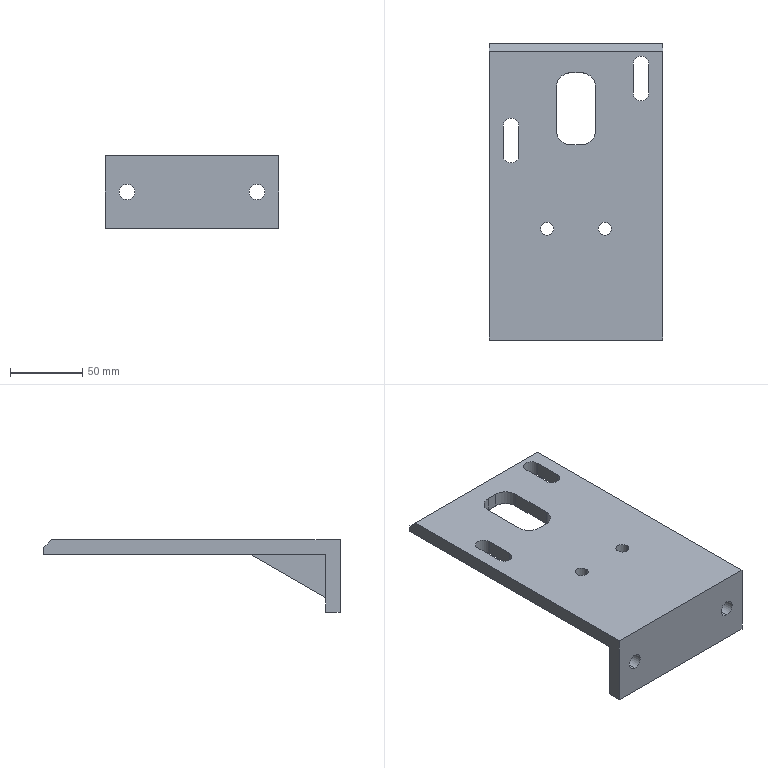NC program | NX | posted with a generic post | part box 120 x 205 x 50 mm
Whole program:
N10 G17 G21 G94 G90
(FLOOR_WALL , TOOL : D80)
N12 T19 M6
N14 G54
N16 G17 G0 G90 X-150.5 Y64.997 B0. C0. S6500 M3
N18 G43 Z30. H19
N20 Z3.
N22 G94 G1 Z0. F1500.
N24 X-147.5
N26 X147.5
N28 Y15.999
N30 X-147.5
N32 Y-33.
N34 X147.5
N36 X150.5
N38 Z3.
N40 G0 Z30.
N42 M5
(ZLEVEL_PROFILE , TOOL : D10)
N44 T15 M6
N46 G54
N48 G17 G0 G90 X-107.6 Y25.993 B0. C0. S9500 M3
N50 G43 Z30. H15
N52 Z1.5
N54 G94 G1 Y60. Z-0.282 F2500.
N56 Y60.554 Z-0.311
N58 X-107.266 Y61.898 Z-0.384
N60 X-106.584 Y63.104 Z-0.456
N62 X-105.604 Y64.084 Z-0.529
N64 X-104.398 Y64.766 Z-0.602
N66 X-103.054 Y65.1 Z-0.674
N68 X-102.5 Z-0.703
N70 X98.203
N72 G2 X103.345 Y60. R5.121
N74 G1 Y-60.
N76 G2 X98.203 Y-65.1 R5.121
N78 G1 X-102.5
N80 G2 X-107.6 Y-60. R5.1
N82 G1 Y60.
N84 G2 X-102.5 Y65.1 R5.1
N86 G1 X-61.99 Z-1.41
N88 X98.91
N90 G2 X104.052 Y60. R5.121
N92 G1 Y-60.
N94 G2 X98.91 Y-65.1 R5.143
N96 G1 X-102.5
N98 G2 X-107.6 Y-60. R5.1
N100 G1 Y60.
N102 G2 X-102.5 Y65.1 R5.1
N104 G1 X-61.99 Z-2.118
N106 X99.618
N108 G2 X104.759 Y60. R5.121
N110 G1 Y-60.
N112 G2 X99.618 Y-65.1 R5.143
N114 G1 X-102.5
N116 G2 X-107.6 Y-60. R5.1
N118 G1 Y60.
N120 G2 X-102.5 Y65.1 R5.1
N122 G1 X-61.99 Z-2.825
N124 X100.325
N126 G2 X105.466 Y60. R5.128
N128 G1 Y-60.
N130 G2 X100.325 Y-65.1 R5.145
N132 G1 X-102.5
N134 G2 X-107.6 Y-60. R5.1
N136 G1 Y60.
N138 G2 X-102.5 Y65.1 R5.1
N140 G1 X-61.99 Z-3.532
N142 X101.032
N144 G2 X106.173 Y60. R5.121
N146 G1 Y-60.
N148 G2 X101.032 Y-65.1 R5.153
N150 G1 X-102.5
N152 G2 X-107.6 Y-60. R5.1
N154 G1 Y60.
N156 G2 X-102.5 Y65.1 R5.1
N158 G1 X-61.99 Z-4.239
N160 X101.739
N162 G2 X106.88 Y60. R5.121
N164 G1 Y-60.
N166 G2 X101.739 Y-65.1 R5.151
N168 G1 X-102.5
N170 G2 X-107.6 Y-60. R5.1
N172 G1 Y60.
N174 G2 X-102.5 Y65.1 R5.1
N176 G1 X-61.634 Z-4.952
N178 X102.452
N180 G2 X107.588 Y60. R5.118
N182 G1 Y-60.
N184 G2 X102.452 Y-65.1 R5.118
N186 G1 X-102.5
N188 G2 X-107.6 Y-60. R5.1
N190 G1 Y60.
N192 G2 X-102.5 Y65.1 R5.1
N194 G1 X-45.245 Z-5.952
N196 X102.5
N198 G2 X107.6 Y60. R5.1
N200 G1 Y-60.
N202 G2 X102.5 Y-65.1 R5.1
N204 G1 X-102.5
N206 G2 X-107.6 Y-60. R5.1
N208 G1 Y60.
N210 G2 X-102.5 Y65.1 R5.1
N212 G1 X-45.21 Z-6.952
N214 X102.5
N216 G2 X107.6 Y60. R5.1
N218 G1 Y-60.
N220 G2 X102.5 Y-65.1 R5.1
N222 G1 X-102.5
N224 G2 X-107.6 Y-60. R5.1
N226 G1 Y60.
N228 G2 X-102.5 Y65.1 R5.1
N230 G1 X-45.21 Z-7.952
N232 X102.5
N234 G2 X107.6 Y60. R5.1
N236 G1 Y-60.
N238 G2 X102.5 Y-65.1 R5.1
N240 G1 X-102.5
N242 G2 X-107.6 Y-60. R5.1
N244 G1 Y60.
N246 G2 X-102.5 Y65.1 R5.1
N248 G1 X-45.21 Z-8.952
N250 X102.5
N252 G2 X107.6 Y60. R5.1
N254 G1 Y-60.
N256 G2 X102.5 Y-65.1 R5.1
N258 G1 X-102.5
N260 G2 X-107.6 Y-60. R5.1
N262 G1 Y60.
N264 G2 X-102.5 Y65.1 R5.1
N266 G1 X-45.21 Z-9.952
N268 X102.5
N270 G2 X107.6 Y60. R5.1
N272 G1 Y-60.
N274 G2 X102.5 Y-65.1 R5.1
N276 G1 X-102.5
N278 G2 X-107.6 Y-60. R5.1
N280 G1 Y60.
N282 G2 X-102.5 Y65.1 R5.1
N284 G1 X-45.21 Z-10.952
N286 X102.5
N288 G2 X107.6 Y60. R5.1
N290 G1 Y-60.
N292 G2 X102.5 Y-65.1 R5.1
N294 G1 X-102.5
N296 G2 X-107.6 Y-60. R5.1
N298 G1 Y60.
N300 G2 X-102.5 Y65.1 R5.1
N302 G1 X-45.21 Z-11.952
N304 X102.5
N306 G2 X107.6 Y60. R5.1
N308 G1 Y-60.
N310 G2 X102.5 Y-65.1 R5.1
N312 G1 X-102.5
N314 G2 X-107.6 Y-60. R5.1
N316 G1 Y60.
N318 G2 X-102.5 Y65.1 R5.1
N320 G1 X-45.21 Z-12.952
N322 X102.5
N324 G2 X107.6 Y60. R5.1
N326 G1 Y-60.
N328 G2 X102.5 Y-65.1 R5.1
N330 G1 X-102.5
N332 G2 X-107.6 Y-60. R5.1
N334 G1 Y60.
N336 G2 X-102.5 Y65.1 R5.1
N338 G1 X-45.21 Z-13.952
N340 X102.5
N342 G2 X107.6 Y60. R5.1
N344 G1 Y-60.
N346 G2 X102.5 Y-65.1 R5.1
N348 G1 X-102.5
N350 G2 X-107.6 Y-60. R5.1
N352 G1 Y60.
N354 G2 X-102.5 Y65.1 R5.1
N356 G1 X-45.21 Z-14.952
N358 X102.5
N360 G2 X107.6 Y60. R5.1
N362 G1 Y-60.
N364 G2 X102.5 Y-65.1 R5.1
N366 G1 X-102.5
N368 G2 X-107.6 Y-60. R5.1
N370 G1 Y60.
N372 G2 X-102.5 Y65.1 R5.1
N374 G1 X-45.21 Z-15.952
N376 X102.5
N378 G2 X107.6 Y60. R5.1
N380 G1 Y-60.
N382 G2 X102.5 Y-65.1 R5.1
N384 G1 X-102.5
N386 G2 X-107.6 Y-60. R5.1
N388 G1 Y60.
N390 G2 X-102.5 Y65.1 R5.1
N392 G1 X-45.21 Z-16.952
N394 X102.5
N396 G2 X107.6 Y60. R5.1
N398 G1 Y-60.
N400 G2 X102.5 Y-65.1 R5.1
N402 G1 X-102.5
N404 G2 X-107.6 Y-60. R5.1
N406 G1 Y60.
N408 G2 X-102.5 Y65.1 R5.1
N410 G1 X-45.21 Z-17.952
N412 X102.5
N414 G2 X107.6 Y60. R5.1
N416 G1 Y-60.
N418 G2 X102.5 Y-65.1 R5.1
N420 G1 X-102.5
N422 G2 X-107.6 Y-60. R5.1
N424 G1 Y60.
N426 G2 X-102.5 Y65.1 R5.1
N428 G1 X-45.21 Z-18.952
N430 X102.5
N432 G2 X107.6 Y60. R5.1
N434 G1 Y-60.
N436 G2 X102.5 Y-65.1 R5.1
N438 G1 X-102.5
N440 G2 X-107.6 Y-60. R5.1
N442 G1 Y60.
N444 G2 X-102.5 Y65.1 R5.1
N446 G1 X-45.21 Z-19.952
N448 X102.5
N450 G2 X107.6 Y60. R5.1
N452 G1 Y-60.
N454 G2 X102.5 Y-65.1 R5.1
N456 G1 X-102.5
N458 G2 X-107.6 Y-60. R5.1
N460 G1 Y60.
N462 G2 X-102.5 Y65.1 R5.1
N464 G1 X-45.21 Z-20.952
N466 X102.5
N468 G2 X107.6 Y60. R5.1
N470 G1 Y-60.
N472 G2 X102.5 Y-65.1 R5.1
N474 G1 X-102.5
N476 G2 X-107.6 Y-60. R5.1
N478 G1 Y60.
N480 G2 X-102.5 Y65.1 R5.1
N482 G1 X-45.21 Z-21.952
N484 X102.5
N486 G2 X107.6 Y60. R5.1
N488 G1 Y-60.
N490 G2 X102.5 Y-65.1 R5.1
N492 G1 X-102.5
N494 G2 X-107.6 Y-60. R5.1
N496 G1 Y60.
N498 G2 X-102.5 Y65.1 R5.1
N500 G1 X-45.21 Z-22.952
N502 X102.5
N504 G2 X107.6 Y60. R5.1
N506 G1 Y-60.
N508 G2 X102.5 Y-65.1 R5.1
N510 G1 X-102.5
N512 G2 X-107.6 Y-60. R5.1
N514 G1 Y60.
N516 G2 X-102.5 Y65.1 R5.1
N518 G1 X-45.21 Z-23.952
N520 X102.5
N522 G2 X107.6 Y60. R5.1
N524 G1 Y-60.
N526 G2 X102.5 Y-65.1 R5.1
N528 G1 X-102.5
N530 G2 X-107.6 Y-60. R5.1
N532 G1 Y60.
N534 G2 X-102.5 Y65.1 R5.1
N536 G1 X-45.21 Z-24.952
N538 X102.5
N540 G2 X107.6 Y60. R5.1
N542 G1 Y-60.
N544 G2 X102.5 Y-65.1 R5.1
N546 G1 X-102.5
N548 G2 X-107.6 Y-60. R5.1
N550 G1 Y60.
N552 G2 X-102.5 Y65.1 R5.1
N554 G1 X-45.21 Z-25.952
N556 X102.5
N558 G2 X107.6 Y60. R5.1
N560 G1 Y-60.
N562 G2 X102.5 Y-65.1 R5.1
N564 G1 X-102.5
N566 G2 X-107.6 Y-60. R5.1
N568 G1 Y60.
N570 G2 X-102.5 Y65.1 R5.1
N572 G1 X-45.21 Z-26.952
N574 X102.5
N576 G2 X107.6 Y60. R5.1
N578 G1 Y-60.
N580 G2 X102.5 Y-65.1 R5.1
N582 G1 X-102.5
N584 G2 X-107.6 Y-60. R5.1
N586 G1 Y60.
N588 G2 X-102.5 Y65.1 R5.1
N590 G1 X-45.21 Z-27.952
N592 X102.5
N594 G2 X107.6 Y60. R5.1
N596 G1 Y-60.
N598 G2 X102.5 Y-65.1 R5.1
N600 G1 X-102.5
N602 G2 X-107.6 Y-60. R5.1
N604 G1 Y60.
N606 G2 X-102.5 Y65.1 R5.1
N608 G1 X-45.21 Z-28.952
N610 X102.5
N612 G2 X107.6 Y60. R5.1
N614 G1 Y-60.
N616 G2 X102.5 Y-65.1 R5.1
N618 G1 X-102.5
N620 G2 X-107.6 Y-60. R5.1
N622 G1 Y60.
N624 G2 X-102.5 Y65.1 R5.1
N626 G1 X-45.21 Z-29.952
N628 X102.5
N630 G2 X107.6 Y60. R5.1
N632 G1 Y-60.
N634 G2 X102.5 Y-65.1 R5.1
N636 G1 X-102.5
N638 G2 X-107.6 Y-60. R5.1
N640 G1 Y60.
N642 G2 X-102.5 Y65.1 R5.1
N644 G1 X-45.21 Z-30.952
N646 X102.5
N648 G2 X107.6 Y60. R5.1
N650 G1 Y-60.
N652 G2 X102.5 Y-65.1 R5.1
N654 G1 X-102.5
N656 G2 X-107.6 Y-60. R5.1
N658 G1 Y60.
N660 G2 X-102.5 Y65.1 R5.1
N662 G1 X-45.21 Z-31.952
N664 X102.5
N666 G2 X107.6 Y60. R5.1
N668 G1 Y-60.
N670 G2 X102.5 Y-65.1 R5.1
N672 G1 X-102.5
N674 G2 X-107.6 Y-60. R5.1
N676 G1 Y60.
N678 G2 X-102.5 Y65.1 R5.1
N680 G1 X-45.21 Z-32.952
N682 X102.5
N684 G2 X107.6 Y60. R5.1
N686 G1 Y-60.
N688 G2 X102.5 Y-65.1 R5.1
N690 G1 X-102.5
N692 G2 X-107.6 Y-60. R5.1
N694 G1 Y60.
N696 G2 X-102.5 Y65.1 R5.1
N698 G1 X-45.21 Z-33.952
N700 X102.5
N702 G2 X107.6 Y60. R5.1
N704 G1 Y-60.
N706 G2 X102.5 Y-65.1 R5.1
N708 G1 X-102.5
N710 G2 X-107.6 Y-60. R5.1
N712 G1 Y60.
N714 G2 X-102.5 Y65.1 R5.1
N716 G1 X-45.21 Z-34.952
N718 X102.5
N720 G2 X107.6 Y60. R5.1
N722 G1 Y-60.
N724 G2 X102.5 Y-65.1 R5.1
N726 G1 X-102.5
N728 G2 X-107.6 Y-60. R5.1
N730 G1 Y60.
N732 G2 X-102.5 Y65.1 R5.1
N734 G1 X-45.21 Z-35.952
N736 X102.5
N738 G2 X107.6 Y60. R5.1
N740 G1 Y-60.
N742 G2 X102.5 Y-65.1 R5.1
N744 G1 X-102.5
N746 G2 X-107.6 Y-60. R5.1
N748 G1 Y60.
N750 G2 X-102.5 Y65.1 R5.1
N752 G1 X-45.21 Z-36.952
N754 X102.5
N756 G2 X107.6 Y60. R5.1
N758 G1 Y-60.
N760 G2 X102.5 Y-65.1 R5.1
N762 G1 X-102.5
N764 G2 X-107.6 Y-60. R5.1
N766 G1 Y60.
N768 G2 X-102.5 Y65.1 R5.1
N770 G1 X-45.21 Z-37.952
N772 X102.5
N774 G2 X107.6 Y60. R5.1
N776 G1 Y-60.
N778 G2 X102.5 Y-65.1 R5.1
N780 G1 X-102.5
N782 G2 X-107.6 Y-60. R5.1
N784 G1 Y60.
N786 G2 X-102.5 Y65.1 R5.1
N788 G1 X-45.21 Z-38.952
N790 X102.5
N792 G2 X107.6 Y60. R5.1
N794 G1 Y-60.
N796 G2 X102.5 Y-65.1 R5.1
N798 G1 X-102.5
N800 G2 X-107.6 Y-60. R5.1
N802 G1 Y60.
N804 G2 X-102.5 Y65.1 R5.1
N806 G1 X-45.21 Z-39.952
N808 X102.5
N810 G2 X107.6 Y60. R5.1
N812 G1 Y-60.
N814 G2 X102.5 Y-65.1 R5.1
N816 G1 X-102.5
N818 G2 X-107.6 Y-60. R5.1
N820 G1 Y60.
N822 G2 X-102.5 Y65.1 R5.1
N824 G1 X-45.21 Z-40.952
N826 X102.5
N828 G2 X107.6 Y60. R5.1
N830 G1 Y-60.
N832 G2 X102.5 Y-65.1 R5.1
N834 G1 X-102.5
N836 G2 X-107.6 Y-60. R5.1
N838 G1 Y60.
N840 G2 X-102.5 Y65.1 R5.1
N842 G1 X-45.21 Z-41.952
N844 X102.5
N846 G2 X107.6 Y60. R5.1
N848 G1 Y-60.
N850 G2 X102.5 Y-65.1 R5.1
N852 G1 X-102.5
N854 G2 X-107.6 Y-60. R5.1
N856 G1 Y60.
N858 G2 X-102.5 Y65.1 R5.1
N860 G1 X-45.21 Z-42.952
N862 X102.5
N864 G2 X107.6 Y60. R5.1
N866 G1 Y-60.
N868 G2 X102.5 Y-65.1 R5.1
N870 G1 X-102.5
N872 G2 X-107.6 Y-60. R5.1
N874 G1 Y60.
N876 G2 X-102.5 Y65.1 R5.1
N878 G1 X-45.21 Z-43.952
N880 X102.5
N882 G2 X107.6 Y60. R5.1
N884 G1 Y-60.
N886 G2 X102.5 Y-65.1 R5.1
N888 G1 X-102.5
N890 G2 X-107.6 Y-60. R5.1
N892 G1 Y60.
N894 G2 X-102.5 Y65.1 R5.1
N896 G1 X-45.21 Z-44.952
N898 X102.5
N900 G2 X107.6 Y60. R5.1
N902 G1 Y-60.
N904 G2 X102.5 Y-65.1 R5.1
N906 G1 X-102.5
N908 G2 X-107.6 Y-60. R5.1
N910 G1 Y60.
N912 G2 X-102.5 Y65.1 R5.1
N914 G1 X-45.21 Z-45.952
N916 X102.5
N918 G2 X107.6 Y60. R5.1
N920 G1 Y-60.
N922 G2 X102.5 Y-65.1 R5.1
N924 G1 X-102.5
N926 G2 X-107.6 Y-60. R5.1
N928 G1 Y60.
N930 G2 X-102.5 Y65.1 R5.1
N932 G1 X-45.21 Z-46.952
N934 X102.5
N936 G2 X107.6 Y60. R5.1
N938 G1 Y-60.
N940 G2 X102.5 Y-65.1 R5.1
N942 G1 X-102.5
N944 G2 X-107.6 Y-60. R5.1
N946 G1 Y60.
N948 G2 X-102.5 Y65.1 R5.1
N950 G1 X-58.839 Z-47.714
N952 X102.5
N954 G2 X107.6 Y60. R5.1
N956 G1 Y-60.
N958 G2 X102.5 Y-65.1 R5.1
N960 G1 X-102.5
N962 G2 X-107.6 Y-60. R5.1
N964 G1 Y60.
N966 G2 X-102.5 Y65.1 R5.1
N968 G1 X-58.839 Z-48.476
N970 X102.5
N972 G2 X107.6 Y60. R5.1
N974 G1 Y-60.
N976 G2 X102.5 Y-65.1 R5.1
N978 G1 X-102.5
N980 G2 X-107.6 Y-60. R5.1
N982 G1 Y60.
N984 G2 X-102.5 Y65.1 R5.1
N986 G1 X-58.839 Z-49.238
N988 X102.5
N990 G2 X107.6 Y60. R5.1
N992 G1 Y-60.
N994 G2 X102.5 Y-65.1 R5.1
N996 G1 X-102.5
N998 G2 X-107.6 Y-60. R5.1
N1000 G1 Y60.
N1002 G2 X-102.5 Y65.1 R5.1
N1004 G1 X-58.839 Z-50.
N1006 X102.5
N1008 G2 X107.6 Y60. R5.1
N1010 G1 Y-60.
N1012 G2 X102.5 Y-65.1 R5.1
N1014 G1 X-102.5
N1016 G2 X-107.6 Y-60. R5.1
N1018 G1 Y60.
N1020 G2 X-102.5 Y65.1 R5.1
N1022 G1 X-58.839
N1024 Z-48.5
N1026 G0 Z30.
(ZLEVEL_PROFILE_COPY , TOOL : D10)
N1028 X72.262 Y-44.6
N1030 Z1.5
N1032 G1 X68.439 Z1.3
N1034 X68.23 Y-44.665 Z1.288
N1036 X68.074 Y-45.062 Z1.266
N1038 X68.231 Y-45.336 Z1.249
N1040 X68.342 Y-45.4 Z1.243
N1042 X68.5 Z1.234
N1044 X88.5 Z0.186
N1046 X88.658 Z0.178
N1048 X88.787 Y-45.32 Z0.17
N1050 X88.928 Y-45.038 Z0.153
N1052 X88.866 Y-44.774 Z0.139
N1054 X88.658 Y-44.6 Z0.125
N1056 X68.439 Z-0.935
N1058 X68.23 Y-44.665 Z-0.946
N1060 X68.074 Y-45.062 Z-0.968
N1062 X68.231 Y-45.336 Z-0.985
N1064 X68.342 Y-45.4 Z-0.992
N1066 X68.5 Z-1.
N1068 X88.5
N1070 G3 X88.9 Y-45. R0.4
N1072 X88.5 Y-44.6 R0.4
N1074 G1 X68.5
N1076 G3 X68.1 Y-45. R0.4
N1078 X68.5 Y-45.4 R0.4
N1080 G1 X88.476 Z-1.627
N1082 X88.813 Y-45.248 Z-1.639
N1084 X88.883 Y-44.886 Z-1.651
N1086 X88.626 Y-44.62 Z-1.663
N1088 X88.244 Y-44.6 Z-1.675
N1090 X77.872 Z-2.
N1092 X68.5
N1094 G3 X68.1 Y-45. R0.4
N1096 X68.5 Y-45.4 R0.4
N1098 G1 X88.476 Z-2.627
N1100 X88.813 Y-45.248 Z-2.639
N1102 X88.883 Y-44.886 Z-2.651
N1104 X88.626 Y-44.62 Z-2.663
N1106 X88.244 Y-44.6 Z-2.675
N1108 X77.872 Z-3.
N1110 X68.5
N1112 G3 X68.1 Y-45. R0.4
N1114 X68.5 Y-45.4 R0.4
N1116 G1 X88.476 Z-3.627
N1118 X88.813 Y-45.248 Z-3.639
N1120 X88.883 Y-44.886 Z-3.651
N1122 X88.626 Y-44.62 Z-3.663
N1124 X88.244 Y-44.6 Z-3.675
N1126 X77.872 Z-4.
N1128 X68.5
N1130 G3 X68.1 Y-45. R0.4
N1132 X68.5 Y-45.4 R0.4
N1134 G1 X88.476 Z-4.627
N1136 X88.813 Y-45.248 Z-4.639
N1138 X88.883 Y-44.886 Z-4.651
N1140 X88.626 Y-44.62 Z-4.663
N1142 X88.244 Y-44.6 Z-4.675
N1144 X77.872 Z-5.
N1146 X68.5
N1148 G3 X68.1 Y-45. R0.4
N1150 X68.5 Y-45.4 R0.4
N1152 G1 X88.476 Z-5.627
N1154 X88.813 Y-45.248 Z-5.639
N1156 X88.883 Y-44.886 Z-5.651
N1158 X88.626 Y-44.62 Z-5.663
N1160 X88.244 Y-44.6 Z-5.675
N1162 X77.872 Z-6.
N1164 X68.5
N1166 G3 X68.1 Y-45. R0.4
N1168 X68.5 Y-45.4 R0.4
N1170 G1 X88.476 Z-6.627
N1172 X88.813 Y-45.248 Z-6.639
N1174 X88.883 Y-44.886 Z-6.651
N1176 X88.626 Y-44.62 Z-6.663
N1178 X88.244 Y-44.6 Z-6.675
N1180 X77.872 Z-7.
N1182 X68.5
N1184 G3 X68.1 Y-45. R0.4
N1186 X68.5 Y-45.4 R0.4
N1188 G1 X88.476 Z-7.627
N1190 X88.813 Y-45.248 Z-7.639
N1192 X88.883 Y-44.886 Z-7.651
N1194 X88.626 Y-44.62 Z-7.663
N1196 X88.244 Y-44.6 Z-7.675
N1198 X77.872 Z-8.
N1200 X68.5
N1202 G3 X68.1 Y-45. R0.4
N1204 X68.5 Y-45.4 R0.4
N1206 G1 X88.476 Z-8.627
N1208 X88.813 Y-45.248 Z-8.639
N1210 X88.883 Y-44.886 Z-8.651
N1212 X88.626 Y-44.62 Z-8.663
N1214 X88.244 Y-44.6 Z-8.675
N1216 X77.872 Z-9.
N1218 X68.5
N1220 G3 X68.1 Y-45. R0.4
N1222 X68.5 Y-45.4 R0.4
N1224 G1 X88.476 Z-9.627
N1226 X88.813 Y-45.248 Z-9.639
N1228 X88.883 Y-44.886 Z-9.651
N1230 X88.626 Y-44.62 Z-9.663
N1232 X88.244 Y-44.6 Z-9.675
N1234 X77.872 Z-10.
N1236 X68.5
N1238 G3 X68.1 Y-45. R0.4
N1240 X68.5 Y-45.4 R0.4
N1242 G1 X88.5
N1244 G3 X88.9 Y-45. R0.4
N1246 X88.5 Y-44.6 R0.4
N1248 G1 X77.872
N1250 Z-8.5
N1252 G0 Z30.
N1254 X41.773 Y44.6
N1256 Z1.5
N1258 G1 X45.658 Z1.296
N1260 X45.872 Y44.784 Z1.282
N1262 X45.926 Y45.062 Z1.267
N1264 X45.769 Y45.336 Z1.25
N1266 X45.658 Y45.4 Z1.244
N1268 X45.5 Z1.235
N1270 X25.5 Z0.187
N1272 X25.342 Z0.179
N1274 X25.231 Y45.336 Z0.172
N1276 X25.074 Y45.062 Z0.156
N1278 X25.073 Y44.952 Z0.15
N1280 X25.221 Y44.673 Z0.133
N1282 X25.342 Y44.6 Z0.126
N1284 X45.658 Z-0.939
N1286 X45.872 Y44.784 Z-0.954
N1288 X45.926 Y45.062 Z-0.968
N1290 X45.769 Y45.336 Z-0.985
N1292 X45.658 Y45.4 Z-0.992
N1294 X45.5 Z-1.
N1296 X25.5
N1298 G3 X25.1 Y45. R0.4
N1300 X25.5 Y44.6 R0.4
N1302 G1 X45.5
N1304 G3 X45.9 Y45. R0.4
N1306 X45.5 Y45.4 R0.4
N1308 G1 X25.524 Z-1.627
N1310 X25.187 Y45.248 Z-1.639
N1312 X25.117 Y44.886 Z-1.651
N1314 X25.374 Y44.62 Z-1.663
N1316 X25.756 Y44.6 Z-1.675
N1318 X36.128 Z-2.
N1320 X45.5
N1322 G3 X45.9 Y45. R0.4
N1324 X45.5 Y45.4 R0.4
N1326 G1 X25.524 Z-2.627
N1328 X25.187 Y45.248 Z-2.639
N1330 X25.117 Y44.886 Z-2.651
N1332 X25.374 Y44.62 Z-2.663
N1334 X25.756 Y44.6 Z-2.675
N1336 X36.128 Z-3.
N1338 X45.5
N1340 G3 X45.9 Y45. R0.4
N1342 X45.5 Y45.4 R0.4
N1344 G1 X25.524 Z-3.627
N1346 X25.187 Y45.248 Z-3.639
N1348 X25.117 Y44.886 Z-3.651
N1350 X25.374 Y44.62 Z-3.663
N1352 X25.756 Y44.6 Z-3.675
N1354 X36.128 Z-4.
N1356 X45.5
N1358 G3 X45.9 Y45. R0.4
N1360 X45.5 Y45.4 R0.4
N1362 G1 X25.524 Z-4.627
N1364 X25.187 Y45.248 Z-4.639
N1366 X25.117 Y44.886 Z-4.651
N1368 X25.374 Y44.62 Z-4.663
N1370 X25.756 Y44.6 Z-4.675
N1372 X36.128 Z-5.
N1374 X45.5
N1376 G3 X45.9 Y45. R0.4
N1378 X45.5 Y45.4 R0.4
N1380 G1 X25.524 Z-5.627
N1382 X25.187 Y45.248 Z-5.639
N1384 X25.117 Y44.886 Z-5.651
N1386 X25.374 Y44.62 Z-5.663
N1388 X25.756 Y44.6 Z-5.675
N1390 X36.128 Z-6.
N1392 X45.5
N1394 G3 X45.9 Y45. R0.4
N1396 X45.5 Y45.4 R0.4
N1398 G1 X25.524 Z-6.627
N1400 X25.187 Y45.248 Z-6.639
N1402 X25.117 Y44.886 Z-6.651
N1404 X25.374 Y44.62 Z-6.663
N1406 X25.756 Y44.6 Z-6.675
N1408 X36.128 Z-7.
N1410 X45.5
N1412 G3 X45.9 Y45. R0.4
N1414 X45.5 Y45.4 R0.4
N1416 G1 X25.524 Z-7.627
N1418 X25.187 Y45.248 Z-7.639
N1420 X25.117 Y44.886 Z-7.651
N1422 X25.374 Y44.62 Z-7.663
N1424 X25.756 Y44.6 Z-7.675
N1426 X36.128 Z-8.
N1428 X45.5
N1430 G3 X45.9 Y45. R0.4
N1432 X45.5 Y45.4 R0.4
N1434 G1 X25.524 Z-8.627
N1436 X25.187 Y45.248 Z-8.639
N1438 X25.117 Y44.886 Z-8.651
N1440 X25.374 Y44.62 Z-8.663
N1442 X25.756 Y44.6 Z-8.675
N1444 X36.128 Z-9.
N1446 X45.5
N1448 G3 X45.9 Y45. R0.4
N1450 X45.5 Y45.4 R0.4
N1452 G1 X25.524 Z-9.627
N1454 X25.187 Y45.248 Z-9.639
N1456 X25.117 Y44.886 Z-9.651
N1458 X25.374 Y44.62 Z-9.663
N1460 X25.756 Y44.6 Z-9.675
N1462 X36.128 Z-10.
N1464 X45.5
N1466 G3 X45.9 Y45. R0.4
N1468 X45.5 Y45.4 R0.4
N1470 G1 X25.5
N1472 G3 X25.1 Y45. R0.4
N1474 X25.5 Y44.6 R0.4
N1476 G1 X36.128
N1478 Z-8.5
N1480 G0 Z30.
(ZLEVEL_PROFILE_COPY_1_COPY_COPY_1 , TOOL : D10JING)
N1482 T14 M6
N1484 G17 G43 G0 G90 X-104.122 Y66.809 Z30. B0. C0. S9500 H14 M3
N1486 Z-15.667
N1488 G94 G1 Z-16.667 F1000.
N1490 X-103.366 Y65.5
N1492 G3 X-102.5 Y65. R1.
N1494 G1 X102.5 F1200.
N1496 G2 X107.5 Y60. R5.
N1498 G1 Y-60.
N1500 G2 X102.5 Y-65. R5.
N1502 G1 X-102.5
N1504 G2 X-107.5 Y-60. R5.
N1506 G1 Y60.
N1508 G2 X-102.5 Y65. R5.
N1510 G3 X-101.634 Y65.5 R1.
N1512 G1 X-100.768 Y67.
N1514 Z-15.667
N1516 G0 Z30.
N1518 X-104.122 Y66.809
N1520 Z-32.333
N1522 G1 Z-33.333 F1000.
N1524 X-103.366 Y65.5
N1526 G3 X-102.5 Y65. R1.
N1528 G1 X102.5 F1200.
N1530 G2 X107.5 Y60. R5.
N1532 G1 Y-60.
N1534 G2 X102.5 Y-65. R5.
N1536 G1 X-102.5
N1538 G2 X-107.5 Y-60. R5.
N1540 G1 Y60.
N1542 G2 X-102.5 Y65. R5.
N1544 G3 X-101.634 Y65.5 R1.
N1546 G1 X-100.768 Y67.
N1548 Z-32.333
N1550 G0 Z30.
N1552 X-104.122 Y66.809
N1554 Z-49.
N1556 G1 Z-50. F1000.
N1558 X-103.366 Y65.5
N1560 G3 X-102.5 Y65. R1.
N1562 G1 X102.5 F1200.
N1564 G2 X107.5 Y60. R5.
N1566 G1 Y-60.
N1568 G2 X102.5 Y-65. R5.
N1570 G1 X-102.5
N1572 G2 X-107.5 Y-60. R5.
N1574 G1 Y60.
N1576 G2 X-102.5 Y65. R5.
N1578 G3 X-101.634 Y65.5 R1.
N1580 G1 X-100.768 Y67.
N1582 Z-49.
N1584 G0 Z30.
N1586 M5
(HOLE_MILLING , TOOL : D6)
N1588 T12 M6
N1590 G54
N1592 G17 G0 G90 X-25.5 Y20. B0. C0. S9500 M3
N1594 G43 Z30. H12
N1596 Z0.5
N1598 G94 G3 X-26.2 Y19.3 R0.7 F1650.
N1600 X-25.5 Y18.6 R0.7
N1602 X-25.5 Y18.6 Z0. I0. J1.4
N1604 X-25.5 Y18.6 Z-0.5 I0. J1.4
N1606 X-25.5 Y18.6 Z-1. I0. J1.4
N1608 X-25.5 Y18.6 Z-1.5 I0. J1.4
N1610 X-25.5 Y18.6 Z-2. I0. J1.4
N1612 X-25.5 Y18.6 Z-2.5 I0. J1.4
N1614 X-25.5 Y18.6 Z-3. I0. J1.4
N1616 X-25.5 Y18.6 Z-3.5 I0. J1.4
N1618 X-25.5 Y18.6 Z-4. I0. J1.4
N1620 X-25.5 Y18.6 Z-4.5 I0. J1.4
N1622 X-25.5 Y18.6 Z-5. I0. J1.4
N1624 X-25.5 Y18.6 Z-5.5 I0. J1.4
N1626 X-25.5 Y18.6 Z-6. I0. J1.4
N1628 X-25.5 Y18.6 Z-6.5 I0. J1.4
N1630 X-25.5 Y18.6 Z-7. I0. J1.4
N1632 X-25.5 Y18.6 Z-7.5 I0. J1.4
N1634 X-25.5 Y18.6 Z-8. I0. J1.4
N1636 X-25.5 Y18.6 Z-8.5 I0. J1.4
N1638 X-25.5 Y18.6 Z-9. I0. J1.4
N1640 X-25.5 Y18.6 Z-9.5 I0. J1.4
N1642 X-25.5 Y18.6 Z-10. I0. J1.4
N1644 X-24.1 Y20. R1.4
N1646 X-25.5 Y18.6 R-1.4
N1648 X-24.8 Y19.3 R0.7
N1650 X-25.5 Y20. R0.7
N1652 G0 Z30.
N1654 Y-20.
N1656 Z0.5
N1658 G3 X-26.2 Y-20.7 R0.7
N1660 X-25.5 Y-21.4 R0.7
N1662 X-25.5 Y-21.4 Z0. I0. J1.4
N1664 X-25.5 Y-21.4 Z-0.5 I0. J1.4
N1666 X-25.5 Y-21.4 Z-1. I0. J1.4
N1668 X-25.5 Y-21.4 Z-1.5 I0. J1.4
N1670 X-25.5 Y-21.4 Z-2. I0. J1.4
N1672 X-25.5 Y-21.4 Z-2.5 I0. J1.4
N1674 X-25.5 Y-21.4 Z-3. I0. J1.4
N1676 X-25.5 Y-21.4 Z-3.5 I0. J1.4
N1678 X-25.5 Y-21.4 Z-4. I0. J1.4
N1680 X-25.5 Y-21.4 Z-4.5 I0. J1.4
N1682 X-25.5 Y-21.4 Z-5. I0. J1.4
N1684 X-25.5 Y-21.4 Z-5.5 I0. J1.4
N1686 X-25.5 Y-21.4 Z-6. I0. J1.4
N1688 X-25.5 Y-21.4 Z-6.5 I0. J1.4
N1690 X-25.5 Y-21.4 Z-7. I0. J1.4
N1692 X-25.5 Y-21.4 Z-7.5 I0. J1.4
N1694 X-25.5 Y-21.4 Z-8. I0. J1.4
N1696 X-25.5 Y-21.4 Z-8.5 I0. J1.4
N1698 X-25.5 Y-21.4 Z-9. I0. J1.4
N1700 X-25.5 Y-21.4 Z-9.5 I0. J1.4
N1702 X-25.5 Y-21.4 Z-10. I0. J1.4
N1704 X-24.1 Y-20. R1.4
N1706 X-25.5 Y-21.4 R-1.4
N1708 X-24.8 Y-20.7 R0.7
N1710 X-25.5 Y-20. R0.7
N1712 G0 Z30.
N1714 M5
(ZLEVEL_PROFILE_1 , TOOL : D4R0.5)
N1716 T17 M6
N1718 G54
N1720 G17 G0 G90 X99.963 Y61.145 B0. C0. S9500 M3
N1722 G43 Z30. H17
N1724 Z1.465
N1726 G94 G1 Z-0.035 F1000.
N1728 X99.442 Y60.844
N1730 G3 X99.242 Y60.498 R0.4
N1732 G1 Y-60.498 F3500.
N1734 X99.26 Z-0.053
N1736 X99.278 Z-0.071
N1738 Y60.498
N1740 X99.295 Z-0.088
N1742 X99.313 Z-0.106
N1744 Y-60.498
N1746 X99.331 Z-0.124
N1748 X99.348 Y-60.499 Z-0.141
N1750 Y60.498
N1752 X99.366 Y60.499 Z-0.159
N1754 X99.384 Z-0.177
N1756 Y60.
N1758 Y-60.
N1760 Y-60.499
N1762 X99.402 Z-0.194
N1764 X99.419 Z-0.212
N1766 Y-60.
N1768 Y60.
N1770 Y60.499
N1772 X99.437 Z-0.23
N1774 X99.455 Z-0.247
N1776 Y60.
N1778 Y-60.
N1780 Y-60.499
N1782 X99.472 Z-0.265
N1784 X99.49 Z-0.283
N1786 Y-60.
N1788 Y60.
N1790 Y60.499
N1792 X99.508 Z-0.301
N1794 X99.525 Z-0.318
N1796 Y60.
N1798 Y-60.
N1800 Y-60.499
N1802 X99.543 Z-0.336
N1804 X99.561 Y-60.5 Z-0.354
N1806 Y-60.
N1808 Y60.
N1810 Y60.5
N1812 X99.578 Z-0.371
N1814 X99.596 Z-0.389
N1816 Y60.
N1818 Y-60.
N1820 Y-60.5
N1822 X99.614 Z-0.407
N1824 X99.631 Z-0.424
N1826 Y-60.
N1828 Y60.
N1830 Y60.5
N1832 X99.649 Z-0.442
N1834 X99.667 Z-0.46
N1836 Y60.
N1838 Y-60.
N1840 Y-60.5
N1842 X99.684 Z-0.477
N1844 X99.702 Z-0.495
N1846 Y-60.
N1848 Y60.
N1850 Y60.5
N1852 X99.72 Z-0.513
N1854 X99.737 Z-0.53
N1856 Y60.
N1858 Y-60.
N1860 Y-60.5
N1862 X99.755 Z-0.548
N1864 X99.773 Z-0.566
N1866 Y-60.
N1868 Y60.
N1870 Y60.5
N1872 X99.79 Z-0.583
N1874 X99.808 Z-0.601
N1876 Y60.
N1878 Y-60.
N1880 Y-60.5
N1882 X99.826 Z-0.619
N1884 X99.843 Z-0.636
N1886 X99.844 Y-60.
N1888 Y60.
N1890 X99.843 Y60.5
N1892 X99.861 Z-0.654
N1894 X99.879 Z-0.672
N1896 Y60.
N1898 Y-60.
N1900 Y-60.5
N1902 X99.897 Z-0.689
N1904 X99.914 Z-0.707
N1906 Y-60.
N1908 Y60.
N1910 Y60.5
N1912 X99.932 Z-0.725
N1914 X99.949 Z-0.742
N1916 X99.95 Y60.
N1918 Y-60.
N1920 X99.949 Y-60.5
N1922 X99.967 Z-0.76
N1924 X99.985 Z-0.778
N1926 Y-60.
N1928 Y60.
N1930 Y60.5
N1932 X100.003 Z-0.795
N1934 X100.02 Z-0.813
N1936 Y60.
N1938 Y-60.
N1940 Y-60.5
N1942 X100.038 Z-0.831
N1944 X100.056 Z-0.849
N1946 Y-60.
N1948 Y60.
N1950 Y60.5
N1952 X100.073 Z-0.866
N1954 X100.091 Z-0.884
N1956 Y60.
N1958 Y-60.
N1960 Y-60.5
N1962 X100.109 Z-0.902
N1964 X100.126 Z-0.919
N1966 Y-60.
N1968 Y60.
N1970 Y60.5
N1972 X100.144 Z-0.937
N1974 X100.162 Z-0.955
N1976 Y60.
N1978 Y-60.
N1980 Y-60.5
N1982 X100.179 Z-0.972
N1984 X100.197 Z-0.99
N1986 Y-60.
N1988 Y60.
N1990 Y60.5
N1992 X100.215 Z-1.008
N1994 X100.232 Z-1.025
N1996 Y60.
N1998 Y-60.
N2000 Y-60.5
N2002 X100.25 Z-1.043
N2004 X100.268 Z-1.061
N2006 Y-60.
N2008 Y60.
N2010 Y60.5
N2012 X100.285 Z-1.078
N2014 X100.303 Z-1.096
N2016 Y60.
N2018 Y-60.
N2020 Y-60.5
N2022 X100.321 Z-1.114
N2024 X100.338 Z-1.131
N2026 Y-60.
N2028 Y60.
N2030 Y60.5
N2032 X100.356 Z-1.149
N2034 X100.374 Z-1.167
N2036 Y60.
N2038 Y-60.
N2040 Y-60.5
N2042 X100.392 Z-1.184
N2044 X100.409 Z-1.202
N2046 Y-60.
N2048 Y60.
N2050 Y60.5
N2052 X100.427 Z-1.22
N2054 X100.444 Z-1.237
N2056 X100.445 Y60.
N2058 Y-60.
N2060 X100.444 Y-60.5
N2062 X100.462 Z-1.255
N2064 X100.48 Z-1.273
N2066 Y-60.
N2068 Y60.
N2070 Y60.5
N2072 X100.498 Z-1.29
N2074 X100.515 Z-1.308
N2076 Y60.
N2078 Y-60.
N2080 Y-60.5
N2082 X100.533 Z-1.326
N2084 X100.551 Z-1.344
N2086 Y-60.
N2088 Y60.
N2090 Y60.5
N2092 X100.568 Z-1.361
N2094 X100.586 Z-1.379
N2096 Y60.
N2098 Y-60.
N2100 Y-60.5
N2102 X100.604 Z-1.397
N2104 X100.621 Z-1.414
N2106 Y-60.
N2108 Y60.
N2110 Y60.5
N2112 X100.639 Z-1.432
N2114 X100.657 Z-1.45
N2116 Y60.
N2118 Y-60.
N2120 Y-60.5
N2122 X100.674 Z-1.467
N2124 X100.692 Z-1.485
N2126 Y-60.
N2128 Y60.
N2130 Y60.5
N2132 X100.71 Z-1.503
N2134 X100.727 Z-1.52
N2136 Y60.
N2138 Y-60.
N2140 Y-60.5
N2142 X100.745 Z-1.538
N2144 X100.763 Z-1.556
N2146 Y-60.
N2148 Y60.
N2150 Y60.5
N2152 X100.78 Z-1.573
N2154 X100.798 Z-1.591
N2156 Y60.
N2158 Y-60.
N2160 Y-60.5
N2162 X100.816 Z-1.609
N2164 X100.833 Z-1.626
N2166 Y-60.
N2168 Y60.
N2170 Y60.5
N2172 X100.851 Z-1.644
N2174 X100.869 Z-1.662
N2176 Y60.
N2178 Y-60.
N2180 Y-60.5
N2182 X100.886 Z-1.679
N2184 X100.904 Z-1.697
N2186 Y-60.
N2188 Y60.
N2190 Y60.5
N2192 X100.922 Z-1.715
N2194 X100.939 Z-1.732
N2196 X100.94 Y60.
N2198 Y-60.
N2200 X100.939 Y-60.5
N2202 X100.957 Z-1.75
N2204 X100.975 Z-1.768
N2206 Y-60.
N2208 Y60.
N2210 Y60.5
N2212 X100.993 Z-1.785
N2214 X101.01 Z-1.803
N2216 Y60.
N2218 Y-60.
N2220 Y-60.5
N2222 X101.028 Z-1.821
N2224 X101.045 Z-1.838
N2226 X101.046 Y-60.
N2228 Y60.
N2230 X101.045 Y60.5
N2232 X101.063 Z-1.856
N2234 X101.081 Z-1.874
N2236 Y60.
N2238 Y-60.
N2240 Y-60.5
N2242 X101.099 Z-1.892
N2244 X101.116 Z-1.909
N2246 Y-60.
N2248 Y60.
N2250 Y60.5
N2252 X101.134 Z-1.927
N2254 X101.152 Z-1.945
N2256 Y60.
N2258 Y-60.
N2260 Y-60.5
N2262 X101.169 Z-1.962
N2264 X101.187 Z-1.98
N2266 Y-60.
N2268 Y60.
N2270 Y60.5
N2272 X101.205 Z-1.998
N2274 X101.222 Z-2.015
N2276 Y60.
N2278 Y-60.
N2280 Y-60.5
N2282 X101.24 Z-2.033
N2284 X101.258 Z-2.051
N2286 Y-60.
N2288 Y60.
N2290 Y60.5
N2292 X101.275 Z-2.068
N2294 X101.293 Z-2.086
N2296 Y60.
N2298 Y-60.
N2300 Y-60.5
N2302 X101.311 Z-2.104
N2304 X101.328 Z-2.121
N2306 Y-60.
N2308 Y60.
N2310 Y60.5
N2312 X101.346 Z-2.139
N2314 X101.364 Z-2.157
N2316 Y60.
N2318 Y-60.
N2320 Y-60.5
N2322 X101.381 Z-2.174
N2324 X101.399 Z-2.192
N2326 Y-60.
N2328 Y60.
N2330 Y60.5
N2332 X101.417 Z-2.21
N2334 X101.434 Z-2.227
N2336 Y60.
N2338 Y-60.
N2340 Y-60.5
N2342 X101.452 Z-2.245
N2344 X101.47 Z-2.263
N2346 Y-60.
N2348 Y60.
N2350 Y60.5
N2352 X101.488 Z-2.28
N2354 X101.505 Z-2.298
N2356 Y60.
N2358 Y-60.
N2360 Y-60.5
N2362 X101.523 Z-2.316
N2364 X101.54 Z-2.333
N2366 X101.541 Y-60.
N2368 Y60.
N2370 X101.54 Y60.5
N2372 X101.558 Z-2.351
N2374 X101.576 Z-2.369
N2376 Y60.
N2378 Y-60.
N2380 Y-60.5
N2382 X101.594 Z-2.386
N2384 X101.611 Z-2.404
N2386 Y-60.
N2388 Y60.
N2390 Y60.5
N2392 X101.629 Z-2.422
N2394 X101.647 Z-2.44
N2396 Y60.
N2398 Y-60.
N2400 Y-60.5
N2402 X101.664 Z-2.457
N2404 X101.682 Z-2.475
N2406 Y-60.
N2408 Y60.
N2410 Y60.5
N2412 X101.7 Z-2.493
N2414 X101.717 Z-2.51
N2416 Y60.
N2418 Y-60.
N2420 Y-60.5
N2422 X101.735 Z-2.528
N2424 X101.753 Z-2.546
N2426 Y-60.
N2428 Y60.
N2430 Y60.5
N2432 X101.77 Z-2.563
N2434 X101.788 Z-2.581
N2436 Y60.
N2438 Y-60.
N2440 Y-60.5
N2442 X101.806 Z-2.599
N2444 X101.823 Z-2.616
N2446 Y-60.
N2448 Y60.
N2450 Y60.5
N2452 X101.841 Z-2.634
N2454 X101.859 Z-2.652
N2456 Y60.
N2458 Y-60.
N2460 Y-60.5
N2462 X101.876 Z-2.669
N2464 X101.894 Z-2.687
N2466 Y-60.
N2468 Y60.
N2470 Y60.5
N2472 X101.912 Z-2.705
N2474 X101.929 Z-2.722
N2476 Y60.
N2478 Y-60.
N2480 Y-60.5
N2482 X101.947 Z-2.74
N2484 X101.965 Z-2.758
N2486 Y-60.
N2488 Y60.
N2490 Y60.5
N2492 X101.983 Z-2.775
N2494 X102. Z-2.793
N2496 Y60.
N2498 Y-60.
N2500 Y-60.5
N2502 X102.018 Z-2.811
N2504 X102.035 Z-2.828
N2506 X102.036 Y-60.
N2508 Y60.
N2510 X102.035 Y60.5
N2512 X102.053 Z-2.846
N2514 X102.071 Z-2.864
N2516 Y60.
N2518 Y-60.
N2520 Y-60.5
N2522 X102.089 Z-2.881
N2524 X102.106 Z-2.899
N2526 Y-60.
N2528 Y60.
N2530 Y60.5
N2532 X102.124 Z-2.917
N2534 X102.142 Z-2.934
N2536 Y60.
N2538 Y-60.
N2540 Y-60.5
N2542 X102.159 Z-2.952
N2544 X102.177 Z-2.97
N2546 Y-60.
N2548 Y60.
N2550 Y60.5
N2552 X102.195 Z-2.988
N2554 X102.212 Z-3.005
N2556 Y60.
N2558 Y-60.
N2560 Y-60.5
N2562 X102.23 Z-3.023
N2564 X102.248 Z-3.041
N2566 Y-60.
N2568 Y60.
N2570 Y60.5
N2572 X102.265 Z-3.058
N2574 X102.283 Z-3.076
N2576 Y60.
N2578 Y-60.
N2580 Y-60.5
N2582 X102.301 Z-3.094
N2584 X102.318 Z-3.111
N2586 Y-60.
N2588 Y60.
N2590 Y60.5
N2592 X102.336 Z-3.129
N2594 X102.354 Z-3.147
N2596 Y60.
N2598 Y-60.
N2600 Y-60.5
N2602 X102.371 Z-3.164
N2604 X102.389 Z-3.182
N2606 Y-60.
N2608 Y60.
N2610 Y60.5
N2612 X102.407 Z-3.2
N2614 X102.424 Z-3.217
N2616 Y60.
N2618 Y-60.
N2620 Y-60.5
N2622 X102.442 Z-3.235
N2624 X102.46 Z-3.253
N2626 Y-60.
N2628 Y60.
N2630 Y60.5
N2632 X102.477 Z-3.27
N2634 X102.495 Z-3.288
N2636 Y60.
N2638 Y-60.
N2640 Y-60.5
N2642 X102.513 Z-3.306
N2644 X102.53 Z-3.323
N2646 X102.531 Y-60.
N2648 Y60.
N2650 X102.53 Y60.5
N2652 X102.548 Z-3.341
N2654 X102.566 Z-3.359
N2656 Y60.
N2658 Y-60.
N2660 Y-60.5
N2662 X102.584 Z-3.376
N2664 X102.601 Z-3.394
N2666 Y-60.
N2668 Y60.
N2670 Y60.5
N2672 X102.619 Z-3.412
N2674 X102.636 Z-3.429
N2676 X102.637 Y60.
N2678 Y-60.
N2680 X102.636 Y-60.5
N2682 X102.654 Z-3.447
N2684 X102.672 Z-3.465
N2686 Y-60.
N2688 Y60.
N2690 Y60.5
N2692 X102.69 Z-3.483
N2694 X102.707 Z-3.5
N2696 Y60.
N2698 Y-60.
N2700 Y-60.5
N2702 X102.725 Z-3.518
N2704 X102.743 Z-3.536
N2706 Y-60.
N2708 Y60.
N2710 Y60.5
N2712 X102.76 Z-3.553
N2714 X102.778 Z-3.571
N2716 Y60.
N2718 Y-60.
N2720 Y-60.5
N2722 X102.796 Z-3.589
N2724 X102.813 Z-3.606
N2726 Y-60.
N2728 Y60.
N2730 Y60.5
N2732 X102.831 Z-3.624
N2734 X102.849 Z-3.642
N2736 Y60.
N2738 Y-60.
N2740 Y-60.5
N2742 X102.866 Z-3.659
N2744 X102.884 Z-3.677
N2746 Y-60.
N2748 Y60.
N2750 Y60.5
N2752 X102.902 Z-3.695
N2754 X102.919 Z-3.712
N2756 Y60.
N2758 Y-60.
N2760 Y-60.5
N2762 X102.937 Z-3.73
N2764 X102.955 Z-3.748
N2766 Y-60.
N2768 Y60.
N2770 Y60.5
N2772 X102.972 Z-3.765
N2774 X102.99 Z-3.783
N2776 Y60.
N2778 Y-60.
N2780 Y-60.5
N2782 X103.008 Z-3.801
N2784 X103.025 Z-3.818
N2786 Y-60.
N2788 Y60.
N2790 Y60.5
N2792 X103.043 Z-3.836
N2794 X103.061 Z-3.854
N2796 Y60.
N2798 Y-60.
N2800 Y-60.5
N2802 X103.079 Z-3.871
N2804 X103.096 Z-3.889
N2806 Y-60.
N2808 Y60.
N2810 Y60.5
N2812 X103.114 Z-3.907
N2814 X103.131 Z-3.924
N2816 X103.132 Y60.
N2818 Y-60.
N2820 X103.131 Y-60.5
N2822 X103.149 Z-3.942
N2824 X103.167 Z-3.96
N2826 Y-60.
N2828 Y60.
N2830 Y60.5
N2832 X103.185 Z-3.977
N2834 X103.202 Z-3.995
N2836 Y60.
N2838 Y-60.
N2840 Y-60.5
N2842 X103.22 Z-4.013
N2844 X103.238 Z-4.031
N2846 Y-60.
N2848 Y60.
N2850 Y60.5
N2852 X103.255 Z-4.048
N2854 X103.273 Z-4.066
N2856 Y60.
N2858 Y-60.
N2860 Y-60.5
N2862 X103.291 Z-4.084
N2864 X103.308 Z-4.101
N2866 Y-60.
N2868 Y60.
N2870 Y60.5
N2872 X103.326 Z-4.119
N2874 X103.344 Z-4.137
N2876 Y60.
N2878 Y-60.
N2880 Y-60.5
N2882 X103.361 Z-4.154
N2884 X103.379 Z-4.172
N2886 Y-60.
N2888 Y60.
N2890 Y60.5
N2892 X103.397 Z-4.19
N2894 X103.414 Z-4.207
N2896 Y60.
N2898 Y-60.
N2900 Y-60.5
N2902 X103.432 Z-4.225
N2904 X103.45 Z-4.243
N2906 Y-60.
N2908 Y60.
N2910 Y60.5
N2912 X103.467 Z-4.26
N2914 X103.485 Z-4.278
N2916 Y60.
N2918 Y-60.
N2920 Y-60.5
N2922 X103.503 Z-4.296
N2924 X103.52 Z-4.313
N2926 Y-60.
N2928 Y60.
N2930 Y60.5
N2932 X103.538 Z-4.331
N2934 X103.556 Z-4.349
N2936 Y60.
N2938 Y-60.
N2940 Y-60.5
N2942 X103.573 Z-4.366
N2944 X103.591 Z-4.384
N2946 Y-60.
N2948 Y60.
N2950 Y60.5
N2952 X103.609 Z-4.402
N2954 X103.626 Z-4.419
N2956 X103.627 Y60.
N2958 Y-60.
N2960 X103.626 Y-60.5
N2962 X103.644 Z-4.437
N2964 X103.662 Z-4.455
N2966 Y-60.
N2968 Y60.
N2970 Y60.5
N2972 X103.68 Z-4.472
N2974 X103.697 Z-4.49
N2976 Y60.
N2978 Y-60.
N2980 Y-60.5
N2982 X103.715 Z-4.508
N2984 X103.733 Z-4.525
N2986 Y-60.
N2988 Y60.
N2990 Y60.5
N2992 X103.75 Z-4.543
N2994 X103.768 Z-4.561
N2996 Y60.
N2998 Y-60.
N3000 Y-60.5
N3002 X103.786 Z-4.579
N3004 X103.803 Z-4.596
N3006 Y-60.
N3008 Y60.
N3010 Y60.5
N3012 X103.821 Z-4.614
N3014 X103.839 Z-4.632
N3016 Y60.
N3018 Y-60.
N3020 Y-60.5
N3022 X103.856 Z-4.649
N3024 X103.874 Z-4.667
N3026 Y-60.
N3028 Y60.
N3030 Y60.5
N3032 X103.892 Z-4.685
N3034 X103.909 Z-4.702
N3036 Y60.
N3038 Y-60.
N3040 Y-60.5
N3042 X103.927 Z-4.72
N3044 X103.945 Z-4.738
N3046 Y-60.
N3048 Y60.
N3050 Y60.5
N3052 X103.962 Z-4.755
N3054 X103.98 Z-4.773
N3056 Y60.
N3058 Y-60.
N3060 Y-60.5
N3062 X103.998 Z-4.791
N3064 X104.015 Z-4.808
N3066 Y-60.
N3068 Y60.
N3070 Y60.5
N3072 X104.033 Z-4.826
N3074 X104.051 Z-4.844
N3076 Y60.
N3078 Y-60.
N3080 Y-60.5
N3082 X104.068 Z-4.861
N3084 X104.086 Z-4.879
N3086 Y-60.
N3088 Y60.
N3090 Y60.5
N3092 X104.104 Z-4.897
N3094 X104.121 Z-4.914
N3096 X104.122 Y60.
N3098 Y-60.
N3100 X104.121 Y-60.5
N3102 X104.139 Z-4.932
N3104 X104.157 Z-4.95
N3106 Y-60.
N3108 Y60.
N3110 Y60.5
N3112 X104.175 Y60.499 Z-4.967
N3114 X104.192 Z-4.985
N3116 Y60.
N3118 Y-60.
N3120 Y-60.499
N3122 X104.21 Z-5.003
N3124 X104.227 Z-5.02
N3126 X104.228 Y-60.
N3128 Y60.
N3130 X104.227 Y60.499
N3132 X104.245 Z-5.038
N3134 X104.263 Z-5.056
N3136 Y60.
N3138 Y-60.
N3140 Y-60.499
N3142 X104.281 Z-5.073
N3144 X104.298 Z-5.091
N3146 Y-60.
N3148 Y60.
N3150 Y60.499
N3152 X104.316 Z-5.109
N3154 X104.334 Z-5.127
N3156 Y60.
N3158 Y-60.
N3160 Y-60.499
N3162 X104.351 Z-5.144
N3164 X104.369 Y-60.498 Z-5.162
N3166 Y60.498
N3168 X104.387 Z-5.18
N3170 X104.404 Z-5.197
N3172 Y-60.498
N3174 X104.422 Z-5.215
N3176 X104.44 Z-5.233
N3178 Y60.498
N3180 X104.457 Z-5.25
N3182 X104.475 Z-5.268
N3184 Y-60.498
N3186 X104.493 Z-5.286
N3188 X104.51 Z-5.303
N3190 Y60.498
N3192 X104.528 Z-5.321
N3194 X104.546 Y60.497 Z-5.339
N3196 Y-60.497
N3198 X104.563 Z-5.356
N3200 X104.581 Z-5.374
N3202 Y60.497
N3204 X104.597 Z-5.39
N3206 X104.613 Z-5.406
N3208 Y-60.497
N3210 X104.628 Z-5.421
N3212 X104.644 Z-5.437
N3214 Y60.497
N3216 X104.66 Z-5.453
N3218 X104.676 Z-5.469
N3220 Y-60.497
N3222 G3 X104.876 Y-60.843 R0.4
N3224 G1 X105.395 Y-61.143
N3226 Z-3.969
N3228 G0 Z30.
N3230 X105.507 Y-59.848
N3232 Z-4.
N3234 G1 Z-5.5 F1000.
N3236 X104.907 Y-59.501
N3238 G2 X104.707 Y-59.155 R0.4
N3240 G1 Y59.155 F3500.
N3242 G2 X104.907 Y59.501 R0.4
N3244 G1 X105.507 Y59.848
N3246 Z-4.
N3248 G0 Z30.
N3250 M5
(PLANAR_MILL_COPY_COPY_COPY_COPY_COPY_COPY_1 , TOOL : D6A45)
N3252 T01 M6
N3254 G54
N3256 G17 G0 G90 X77.634 Y-49.1 B0. C0. S9500 M3
N3258 G43 Z30. H1
N3260 Z0.5
N3262 G94 G1 Z-1. F1250.
N3264 G3 X78.5 Y-49.6 R1.
N3266 G1 X88.5
N3268 G3 X93.1 Y-45. R4.6
N3270 X88.5 Y-40.4 R4.6
N3272 G1 X68.5
N3274 G3 X63.9 Y-45. R4.6
N3276 X68.5 Y-49.6 R4.6
N3278 G1 X78.5
N3280 G3 X79.366 Y-49.1 R1.
N3282 G1 Z0.5
N3284 G0 Z30.
N3286 X56.634 Y-12.1
N3288 Z0.5
N3290 G1 Z-1.
N3292 G3 X57.5 Y-12.6 R1.
N3294 G1 X72.5
N3296 G3 X81.6 Y-3.5 R9.1
N3298 G1 Y3.5
N3300 G3 X72.5 Y12.6 R9.1
N3302 G1 X42.5
N3304 G3 X33.4 Y3.5 R9.1
N3306 G1 Y-3.5
N3308 G3 X42.5 Y-12.6 R9.1
N3310 G1 X57.5
N3312 G3 X58.366 Y-12.1 R1.
N3314 G1 Z0.5
N3316 G0 Z30.
N3318 X36.366 Y49.1
N3320 Z0.5
N3322 G1 Z-1.
N3324 G3 X35.5 Y49.6 R1.
N3326 G1 X25.5
N3328 G3 X20.9 Y45. R4.6
N3330 X25.5 Y40.4 R4.6
N3332 G1 X45.5
N3334 G3 X50.1 Y45. R4.6
N3336 X45.5 Y49.6 R4.6
N3338 G1 X35.5
N3340 G3 X34.634 Y49.1 R1.
N3342 G1 Z0.5
N3344 G0 Z30.
N3346 X-0.866 Y61.4
N3348 Z0.5
N3350 G1 Z-1.
N3352 G3 X0. Y60.9 R1.
N3354 G1 X102.5
N3356 G2 X103.4 Y60. R0.9
N3358 G1 Y-60.
N3360 G2 X102.5 Y-60.9 R0.9
N3362 G1 X-102.5
N3364 G2 X-103.4 Y-60. R0.9
N3366 G1 Y60.
N3368 G2 X-102.5 Y60.9 R0.9
N3370 G1 X0.
N3372 G3 X0.866 Y61.4 R1.
N3374 G1 Z0.5
N3376 G0 Z30.
N3378 X-24.634 Y23.1
N3380 Z0.5
N3382 G1 Z-1.
N3384 G3 X-25.5 Y23.6 R1.
N3386 X-29.1 Y20. R3.6
N3388 X-25.5 Y23.6 R-3.6
N3390 X-26.366 Y23.1 R1.
N3392 G1 Z0.5
N3394 G0 Z30.
N3396 Y-23.1
N3398 Z0.5
N3400 G1 Z-1.
N3402 G3 X-25.5 Y-23.6 R1.
N3404 X-21.9 Y-20. R3.6
N3406 X-25.5 Y-23.6 R-3.6
N3408 X-24.634 Y-23.1 R1.
N3410 G1 Z0.5
N3412 G0 Z30.
N3414 M5
(刀补6 , TOOL : D6)
N3416 T12 M6
N3418 G54
N3420 G17 G0 G90 X-25.5 Y20. B0. C0. S9500 M3
N3422 G43 Z30. H12
N3424 Z0.5
N3426 G41 G94 G1 X-25.6 Y20.004 F1000. D12
N3428 G3 X-25.5 Y18.55 R0.73
N3430 X-25.5 Y18.55 Z-1.5 I0. J1.45
N3432 X-25.5 Y18.55 Z-3.5 I0. J1.45
N3434 X-25.5 Y18.55 Z-5.5 I0. J1.45
N3436 X-25.5 Y18.55 Z-7.5 I0. J1.45
N3438 X-25.5 Y18.55 Z-9.5 I0. J1.45
N3440 X-24.05 Y20. Z-10. R1.45
N3442 X-25.5 Y21.45 R1.45
N3444 X-24.05 Y20. R-1.45
N3446 X-25.504 Y20.1 R0.73
N3448 G40
N3450 G1 X-25.5 Y20.
N3452 G0 Z30.
N3454 Y-20.
N3456 Z0.5
N3458 G41 G1 X-25.6 Y-19.996
N3460 G3 X-25.5 Y-21.45 R0.73
N3462 X-25.5 Y-21.45 Z-1.5 I0. J1.45
N3464 X-25.5 Y-21.45 Z-3.5 I0. J1.45
N3466 X-25.5 Y-21.45 Z-5.5 I0. J1.45
N3468 X-25.5 Y-21.45 Z-7.5 I0. J1.45
N3470 X-25.5 Y-21.45 Z-9.5 I0. J1.45
N3472 X-24.05 Y-20. Z-10. R1.45
N3474 X-25.5 Y-18.55 R1.45
N3476 X-24.05 Y-20. R-1.45
N3478 X-25.504 Y-19.9 R0.73
N3480 G40
N3482 G1 X-25.5 Y-20.
N3484 G0 Z30.
N3486 M5
N3488 M2